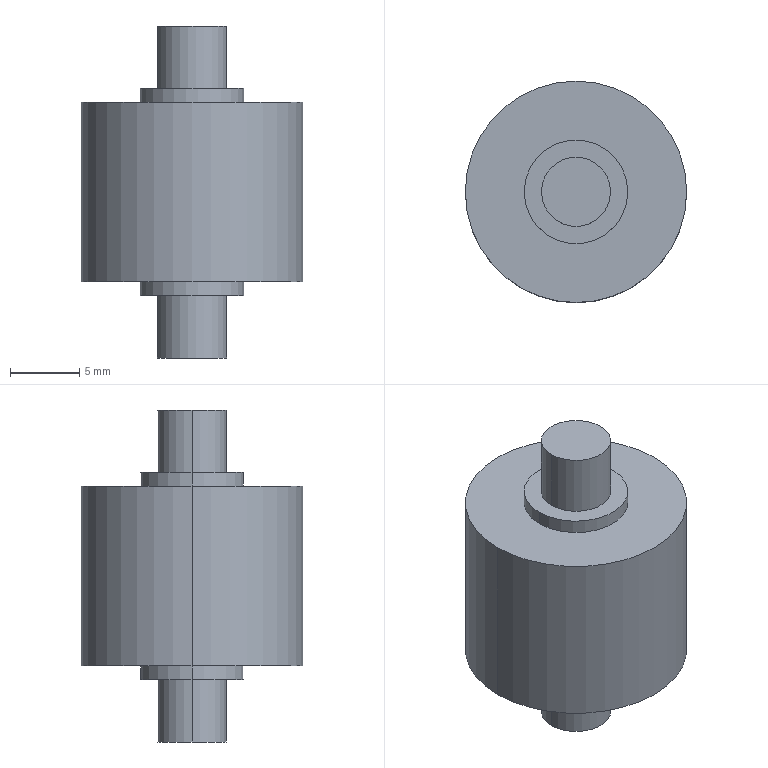Part | 1 solid | 16 faces | box 16 x 16 x 24 mm | volume 2879 mm3 | cylinder 10 | plane 6 | commonest cylinder face diameters 5 x4 7.5 x4 16 x2
STEP:
#1=CARTESIAN_POINT('',(2.5,0.,12.));
#2=VERTEX_POINT('',#1);
#3=CARTESIAN_POINT('',(-2.5,0.,12.));
#4=VERTEX_POINT('',#3);
#5=CARTESIAN_POINT('',(0.,0.,12.));
#6=DIRECTION('',(0.,0.,1.));
#7=DIRECTION('',(1.,0.,0.));
#8=AXIS2_PLACEMENT_3D('',#5,#6,#7);
#9=CIRCLE('',#8,2.5);
#10=EDGE_CURVE('',#2,#4,#9,.T.);
#11=ORIENTED_EDGE('',*,*,#10,.F.);
#12=CARTESIAN_POINT('',(2.5,0.,7.5));
#13=VERTEX_POINT('',#12);
#14=CARTESIAN_POINT('',(2.5,0.,12.));
#15=DIRECTION('',(0.,0.,-1.));
#16=VECTOR('',#15,1000.);
#17=LINE('',#14,#16);
#18=EDGE_CURVE('',#2,#13,#17,.T.);
#19=ORIENTED_EDGE('',*,*,#18,.T.);
#20=CARTESIAN_POINT('',(-2.5,0.,7.5));
#21=VERTEX_POINT('',#20);
#22=CARTESIAN_POINT('',(0.,0.,7.5));
#23=DIRECTION('',(0.,0.,1.));
#24=DIRECTION('',(1.,0.,0.));
#25=AXIS2_PLACEMENT_3D('',#22,#23,#24);
#26=CIRCLE('',#25,2.5);
#27=EDGE_CURVE('',#13,#21,#26,.T.);
#28=ORIENTED_EDGE('',*,*,#27,.T.);
#29=CARTESIAN_POINT('',(-2.5,0.,12.));
#30=DIRECTION('',(0.,0.,-1.));
#31=VECTOR('',#30,1000.);
#32=LINE('',#29,#31);
#33=EDGE_CURVE('',#4,#21,#32,.T.);
#34=ORIENTED_EDGE('',*,*,#33,.F.);
#35=EDGE_LOOP('',(#11,#19,#28,#34));
#36=FACE_OUTER_BOUND('',#35,.T.);
#37=CARTESIAN_POINT('',(0.,0.,12.));
#38=DIRECTION('',(0.,0.,-1.));
#39=DIRECTION('',(-1.,0.,0.));
#40=AXIS2_PLACEMENT_3D('',#37,#38,#39);
#41=CYLINDRICAL_SURFACE('',#40,2.5);
#42=ADVANCED_FACE('',(#36),#41,.T.);
#43=CARTESIAN_POINT('',(3.75,0.,7.5));
#44=VERTEX_POINT('',#43);
#45=CARTESIAN_POINT('',(-3.75,0.,7.5));
#46=VERTEX_POINT('',#45);
#47=CARTESIAN_POINT('',(0.,0.,7.5));
#48=DIRECTION('',(0.,0.,1.));
#49=DIRECTION('',(1.,0.,0.));
#50=AXIS2_PLACEMENT_3D('',#47,#48,#49);
#51=CIRCLE('',#50,3.75);
#52=EDGE_CURVE('',#44,#46,#51,.T.);
#53=ORIENTED_EDGE('',*,*,#52,.F.);
#54=CARTESIAN_POINT('',(3.75,0.,6.5));
#55=VERTEX_POINT('',#54);
#56=CARTESIAN_POINT('',(3.75,0.,7.5));
#57=DIRECTION('',(0.,0.,-1.));
#58=VECTOR('',#57,1000.);
#59=LINE('',#56,#58);
#60=EDGE_CURVE('',#44,#55,#59,.T.);
#61=ORIENTED_EDGE('',*,*,#60,.T.);
#62=CARTESIAN_POINT('',(-3.75,0.,6.5));
#63=VERTEX_POINT('',#62);
#64=CARTESIAN_POINT('',(0.,0.,6.5));
#65=DIRECTION('',(0.,0.,1.));
#66=DIRECTION('',(1.,0.,0.));
#67=AXIS2_PLACEMENT_3D('',#64,#65,#66);
#68=CIRCLE('',#67,3.75);
#69=EDGE_CURVE('',#55,#63,#68,.T.);
#70=ORIENTED_EDGE('',*,*,#69,.T.);
#71=CARTESIAN_POINT('',(-3.75,0.,7.5));
#72=DIRECTION('',(0.,0.,-1.));
#73=VECTOR('',#72,1000.);
#74=LINE('',#71,#73);
#75=EDGE_CURVE('',#46,#63,#74,.T.);
#76=ORIENTED_EDGE('',*,*,#75,.F.);
#77=EDGE_LOOP('',(#53,#61,#70,#76));
#78=FACE_OUTER_BOUND('',#77,.T.);
#79=CARTESIAN_POINT('',(0.,0.,7.5));
#80=DIRECTION('',(0.,0.,-1.));
#81=DIRECTION('',(-1.,0.,0.));
#82=AXIS2_PLACEMENT_3D('',#79,#80,#81);
#83=CYLINDRICAL_SURFACE('',#82,3.75);
#84=ADVANCED_FACE('',(#78),#83,.T.);
#85=CARTESIAN_POINT('',(-2.5,0.,-7.5));
#86=VERTEX_POINT('',#85);
#87=CARTESIAN_POINT('',(2.5,0.,-7.5));
#88=VERTEX_POINT('',#87);
#89=CARTESIAN_POINT('',(0.,0.,-7.5));
#90=DIRECTION('',(0.,0.,-1.));
#91=DIRECTION('',(-1.,0.,0.));
#92=AXIS2_PLACEMENT_3D('',#89,#90,#91);
#93=CIRCLE('',#92,2.5);
#94=EDGE_CURVE('',#86,#88,#93,.T.);
#95=ORIENTED_EDGE('',*,*,#94,.T.);
#96=CARTESIAN_POINT('',(2.5,0.,-12.));
#97=VERTEX_POINT('',#96);
#98=CARTESIAN_POINT('',(2.5,0.,12.));
#99=DIRECTION('',(0.,0.,-1.));
#100=VECTOR('',#99,1000.);
#101=LINE('',#98,#100);
#102=EDGE_CURVE('',#88,#97,#101,.T.);
#103=ORIENTED_EDGE('',*,*,#102,.T.);
#104=CARTESIAN_POINT('',(-2.5,0.,-12.));
#105=VERTEX_POINT('',#104);
#106=CARTESIAN_POINT('',(0.,0.,-12.));
#107=DIRECTION('',(0.,0.,1.));
#108=DIRECTION('',(1.,0.,0.));
#109=AXIS2_PLACEMENT_3D('',#106,#107,#108);
#110=CIRCLE('',#109,2.5);
#111=EDGE_CURVE('',#97,#105,#110,.T.);
#112=ORIENTED_EDGE('',*,*,#111,.T.);
#113=CARTESIAN_POINT('',(-2.5,0.,12.));
#114=DIRECTION('',(0.,0.,-1.));
#115=VECTOR('',#114,1000.);
#116=LINE('',#113,#115);
#117=EDGE_CURVE('',#86,#105,#116,.T.);
#118=ORIENTED_EDGE('',*,*,#117,.F.);
#119=EDGE_LOOP('',(#95,#103,#112,#118));
#120=FACE_OUTER_BOUND('',#119,.T.);
#121=CARTESIAN_POINT('',(0.,0.,12.));
#122=DIRECTION('',(0.,0.,-1.));
#123=DIRECTION('',(-1.,0.,0.));
#124=AXIS2_PLACEMENT_3D('',#121,#122,#123);
#125=CYLINDRICAL_SURFACE('',#124,2.5);
#126=ADVANCED_FACE('',(#120),#125,.T.);
#127=CARTESIAN_POINT('',(-3.75,0.,-7.5));
#128=VERTEX_POINT('',#127);
#129=CARTESIAN_POINT('',(3.75,0.,-7.5));
#130=VERTEX_POINT('',#129);
#131=CARTESIAN_POINT('',(0.,0.,-7.5));
#132=DIRECTION('',(0.,0.,-1.));
#133=DIRECTION('',(-1.,0.,0.));
#134=AXIS2_PLACEMENT_3D('',#131,#132,#133);
#135=CIRCLE('',#134,3.75);
#136=EDGE_CURVE('',#128,#130,#135,.T.);
#137=ORIENTED_EDGE('',*,*,#136,.F.);
#138=CARTESIAN_POINT('',(-3.75,0.,-6.5));
#139=VERTEX_POINT('',#138);
#140=CARTESIAN_POINT('',(-3.75,0.,-7.5));
#141=DIRECTION('',(0.,0.,1.));
#142=VECTOR('',#141,1000.);
#143=LINE('',#140,#142);
#144=EDGE_CURVE('',#128,#139,#143,.T.);
#145=ORIENTED_EDGE('',*,*,#144,.T.);
#146=CARTESIAN_POINT('',(3.75,0.,-6.5));
#147=VERTEX_POINT('',#146);
#148=CARTESIAN_POINT('',(0.,0.,-6.5));
#149=DIRECTION('',(0.,0.,-1.));
#150=DIRECTION('',(1.,0.,0.));
#151=AXIS2_PLACEMENT_3D('',#148,#149,#150);
#152=CIRCLE('',#151,3.75);
#153=EDGE_CURVE('',#139,#147,#152,.T.);
#154=ORIENTED_EDGE('',*,*,#153,.T.);
#155=CARTESIAN_POINT('',(3.75,0.,-7.5));
#156=DIRECTION('',(0.,0.,1.));
#157=VECTOR('',#156,1000.);
#158=LINE('',#155,#157);
#159=EDGE_CURVE('',#130,#147,#158,.T.);
#160=ORIENTED_EDGE('',*,*,#159,.F.);
#161=EDGE_LOOP('',(#137,#145,#154,#160));
#162=FACE_OUTER_BOUND('',#161,.T.);
#163=CARTESIAN_POINT('',(0.,0.,-7.5));
#164=DIRECTION('',(0.,0.,1.));
#165=DIRECTION('',(1.,0.,0.));
#166=AXIS2_PLACEMENT_3D('',#163,#164,#165);
#167=CYLINDRICAL_SURFACE('',#166,3.75);
#168=ADVANCED_FACE('',(#162),#167,.T.);
#169=CARTESIAN_POINT('',(8.,0.,6.5));
#170=VERTEX_POINT('',#169);
#171=CARTESIAN_POINT('',(-8.,0.,6.5));
#172=VERTEX_POINT('',#171);
#173=CARTESIAN_POINT('',(0.,0.,6.5));
#174=DIRECTION('',(0.,0.,1.));
#175=DIRECTION('',(1.,0.,0.));
#176=AXIS2_PLACEMENT_3D('',#173,#174,#175);
#177=CIRCLE('',#176,8.);
#178=EDGE_CURVE('',#170,#172,#177,.T.);
#179=ORIENTED_EDGE('',*,*,#178,.F.);
#180=CARTESIAN_POINT('',(8.,0.,-6.5));
#181=VERTEX_POINT('',#180);
#182=CARTESIAN_POINT('',(8.,0.,6.5));
#183=DIRECTION('',(0.,0.,-1.));
#184=VECTOR('',#183,1000.);
#185=LINE('',#182,#184);
#186=EDGE_CURVE('',#170,#181,#185,.T.);
#187=ORIENTED_EDGE('',*,*,#186,.T.);
#188=CARTESIAN_POINT('',(-8.,0.,-6.5));
#189=VERTEX_POINT('',#188);
#190=CARTESIAN_POINT('',(0.,0.,-6.5));
#191=DIRECTION('',(0.,0.,1.));
#192=DIRECTION('',(1.,0.,0.));
#193=AXIS2_PLACEMENT_3D('',#190,#191,#192);
#194=CIRCLE('',#193,8.);
#195=EDGE_CURVE('',#181,#189,#194,.T.);
#196=ORIENTED_EDGE('',*,*,#195,.T.);
#197=CARTESIAN_POINT('',(-8.,0.,6.5));
#198=DIRECTION('',(0.,0.,-1.));
#199=VECTOR('',#198,1000.);
#200=LINE('',#197,#199);
#201=EDGE_CURVE('',#172,#189,#200,.T.);
#202=ORIENTED_EDGE('',*,*,#201,.F.);
#203=EDGE_LOOP('',(#179,#187,#196,#202));
#204=FACE_OUTER_BOUND('',#203,.T.);
#205=CARTESIAN_POINT('',(0.,0.,6.5));
#206=DIRECTION('',(0.,0.,-1.));
#207=DIRECTION('',(-1.,0.,0.));
#208=AXIS2_PLACEMENT_3D('',#205,#206,#207);
#209=CYLINDRICAL_SURFACE('',#208,8.);
#210=ADVANCED_FACE('',(#204),#209,.T.);
#211=ORIENTED_EDGE('',*,*,#186,.F.);
#212=CARTESIAN_POINT('',(0.,0.,6.5));
#213=DIRECTION('',(0.,0.,1.));
#214=DIRECTION('',(1.,0.,0.));
#215=AXIS2_PLACEMENT_3D('',#212,#213,#214);
#216=CIRCLE('',#215,8.);
#217=EDGE_CURVE('',#172,#170,#216,.T.);
#218=ORIENTED_EDGE('',*,*,#217,.F.);
#219=ORIENTED_EDGE('',*,*,#201,.T.);
#220=CARTESIAN_POINT('',(0.,0.,-6.5));
#221=DIRECTION('',(0.,0.,1.));
#222=DIRECTION('',(1.,0.,0.));
#223=AXIS2_PLACEMENT_3D('',#220,#221,#222);
#224=CIRCLE('',#223,8.);
#225=EDGE_CURVE('',#189,#181,#224,.T.);
#226=ORIENTED_EDGE('',*,*,#225,.T.);
#227=EDGE_LOOP('',(#211,#218,#219,#226));
#228=FACE_OUTER_BOUND('',#227,.T.);
#229=CARTESIAN_POINT('',(0.,0.,6.5));
#230=DIRECTION('',(0.,0.,-1.));
#231=DIRECTION('',(-1.,0.,0.));
#232=AXIS2_PLACEMENT_3D('',#229,#230,#231);
#233=CYLINDRICAL_SURFACE('',#232,8.);
#234=ADVANCED_FACE('',(#228),#233,.T.);
#235=CARTESIAN_POINT('',(0.,0.,6.5));
#236=DIRECTION('',(0.,0.,1.));
#237=DIRECTION('',(1.,0.,0.));
#238=AXIS2_PLACEMENT_3D('',#235,#236,#237);
#239=CIRCLE('',#238,3.75);
#240=EDGE_CURVE('',#63,#55,#239,.T.);
#241=ORIENTED_EDGE('',*,*,#240,.F.);
#242=ORIENTED_EDGE('',*,*,#69,.F.);
#243=EDGE_LOOP('',(#241,#242));
#244=FACE_BOUND('',#243,.T.);
#245=ORIENTED_EDGE('',*,*,#217,.T.);
#246=ORIENTED_EDGE('',*,*,#178,.T.);
#247=EDGE_LOOP('',(#245,#246));
#248=FACE_OUTER_BOUND('',#247,.T.);
#249=CARTESIAN_POINT('',(0.,0.,6.5));
#250=DIRECTION('',(0.,0.,1.));
#251=DIRECTION('',(1.,0.,0.));
#252=AXIS2_PLACEMENT_3D('',#249,#250,#251);
#253=PLANE('',#252);
#254=ADVANCED_FACE('',(#244,#248),#253,.T.);
#255=CARTESIAN_POINT('',(0.,0.,-6.5));
#256=DIRECTION('',(0.,0.,-1.));
#257=DIRECTION('',(1.,0.,0.));
#258=AXIS2_PLACEMENT_3D('',#255,#256,#257);
#259=CIRCLE('',#258,3.75);
#260=EDGE_CURVE('',#147,#139,#259,.T.);
#261=ORIENTED_EDGE('',*,*,#260,.F.);
#262=ORIENTED_EDGE('',*,*,#153,.F.);
#263=EDGE_LOOP('',(#261,#262));
#264=FACE_BOUND('',#263,.T.);
#265=ORIENTED_EDGE('',*,*,#225,.F.);
#266=ORIENTED_EDGE('',*,*,#195,.F.);
#267=EDGE_LOOP('',(#265,#266));
#268=FACE_OUTER_BOUND('',#267,.T.);
#269=CARTESIAN_POINT('',(0.,0.,-6.5));
#270=DIRECTION('',(0.,0.,1.));
#271=DIRECTION('',(1.,0.,0.));
#272=AXIS2_PLACEMENT_3D('',#269,#270,#271);
#273=PLANE('',#272);
#274=ADVANCED_FACE('',(#264,#268),#273,.F.);
#275=ORIENTED_EDGE('',*,*,#144,.F.);
#276=CARTESIAN_POINT('',(0.,0.,-7.5));
#277=DIRECTION('',(0.,0.,-1.));
#278=DIRECTION('',(-1.,0.,0.));
#279=AXIS2_PLACEMENT_3D('',#276,#277,#278);
#280=CIRCLE('',#279,3.75);
#281=EDGE_CURVE('',#130,#128,#280,.T.);
#282=ORIENTED_EDGE('',*,*,#281,.F.);
#283=ORIENTED_EDGE('',*,*,#159,.T.);
#284=ORIENTED_EDGE('',*,*,#260,.T.);
#285=EDGE_LOOP('',(#275,#282,#283,#284));
#286=FACE_OUTER_BOUND('',#285,.T.);
#287=CARTESIAN_POINT('',(0.,0.,-7.5));
#288=DIRECTION('',(0.,0.,1.));
#289=DIRECTION('',(1.,0.,0.));
#290=AXIS2_PLACEMENT_3D('',#287,#288,#289);
#291=CYLINDRICAL_SURFACE('',#290,3.75);
#292=ADVANCED_FACE('',(#286),#291,.T.);
#293=ORIENTED_EDGE('',*,*,#94,.F.);
#294=CARTESIAN_POINT('',(0.,0.,-7.5));
#295=DIRECTION('',(0.,0.,-1.));
#296=DIRECTION('',(-1.,0.,0.));
#297=AXIS2_PLACEMENT_3D('',#294,#295,#296);
#298=CIRCLE('',#297,2.5);
#299=EDGE_CURVE('',#88,#86,#298,.T.);
#300=ORIENTED_EDGE('',*,*,#299,.F.);
#301=EDGE_LOOP('',(#293,#300));
#302=FACE_BOUND('',#301,.T.);
#303=ORIENTED_EDGE('',*,*,#281,.T.);
#304=ORIENTED_EDGE('',*,*,#136,.T.);
#305=EDGE_LOOP('',(#303,#304));
#306=FACE_OUTER_BOUND('',#305,.T.);
#307=CARTESIAN_POINT('',(0.,0.,-7.5));
#308=DIRECTION('',(0.,0.,-1.));
#309=DIRECTION('',(-1.,0.,0.));
#310=AXIS2_PLACEMENT_3D('',#307,#308,#309);
#311=PLANE('',#310);
#312=ADVANCED_FACE('',(#302,#306),#311,.T.);
#313=CARTESIAN_POINT('',(0.,0.,-12.));
#314=DIRECTION('',(0.,0.,1.));
#315=DIRECTION('',(1.,0.,0.));
#316=AXIS2_PLACEMENT_3D('',#313,#314,#315);
#317=CIRCLE('',#316,2.5);
#318=EDGE_CURVE('',#105,#97,#317,.T.);
#319=ORIENTED_EDGE('',*,*,#318,.F.);
#320=ORIENTED_EDGE('',*,*,#111,.F.);
#321=EDGE_LOOP('',(#319,#320));
#322=FACE_OUTER_BOUND('',#321,.T.);
#323=CARTESIAN_POINT('',(0.,0.,-12.));
#324=DIRECTION('',(0.,0.,1.));
#325=DIRECTION('',(1.,0.,0.));
#326=AXIS2_PLACEMENT_3D('',#323,#324,#325);
#327=PLANE('',#326);
#328=ADVANCED_FACE('',(#322),#327,.F.);
#329=ORIENTED_EDGE('',*,*,#102,.F.);
#330=ORIENTED_EDGE('',*,*,#299,.T.);
#331=ORIENTED_EDGE('',*,*,#117,.T.);
#332=ORIENTED_EDGE('',*,*,#318,.T.);
#333=EDGE_LOOP('',(#329,#330,#331,#332));
#334=FACE_OUTER_BOUND('',#333,.T.);
#335=CARTESIAN_POINT('',(0.,0.,12.));
#336=DIRECTION('',(0.,0.,-1.));
#337=DIRECTION('',(-1.,0.,0.));
#338=AXIS2_PLACEMENT_3D('',#335,#336,#337);
#339=CYLINDRICAL_SURFACE('',#338,2.5);
#340=ADVANCED_FACE('',(#334),#339,.T.);
#341=ORIENTED_EDGE('',*,*,#60,.F.);
#342=CARTESIAN_POINT('',(0.,0.,7.5));
#343=DIRECTION('',(0.,0.,1.));
#344=DIRECTION('',(1.,0.,0.));
#345=AXIS2_PLACEMENT_3D('',#342,#343,#344);
#346=CIRCLE('',#345,3.75);
#347=EDGE_CURVE('',#46,#44,#346,.T.);
#348=ORIENTED_EDGE('',*,*,#347,.F.);
#349=ORIENTED_EDGE('',*,*,#75,.T.);
#350=ORIENTED_EDGE('',*,*,#240,.T.);
#351=EDGE_LOOP('',(#341,#348,#349,#350));
#352=FACE_OUTER_BOUND('',#351,.T.);
#353=CARTESIAN_POINT('',(0.,0.,7.5));
#354=DIRECTION('',(0.,0.,-1.));
#355=DIRECTION('',(-1.,0.,0.));
#356=AXIS2_PLACEMENT_3D('',#353,#354,#355);
#357=CYLINDRICAL_SURFACE('',#356,3.75);
#358=ADVANCED_FACE('',(#352),#357,.T.);
#359=CARTESIAN_POINT('',(0.,0.,7.5));
#360=DIRECTION('',(0.,0.,1.));
#361=DIRECTION('',(1.,0.,0.));
#362=AXIS2_PLACEMENT_3D('',#359,#360,#361);
#363=CIRCLE('',#362,2.5);
#364=EDGE_CURVE('',#21,#13,#363,.T.);
#365=ORIENTED_EDGE('',*,*,#364,.F.);
#366=ORIENTED_EDGE('',*,*,#27,.F.);
#367=EDGE_LOOP('',(#365,#366));
#368=FACE_BOUND('',#367,.T.);
#369=ORIENTED_EDGE('',*,*,#347,.T.);
#370=ORIENTED_EDGE('',*,*,#52,.T.);
#371=EDGE_LOOP('',(#369,#370));
#372=FACE_OUTER_BOUND('',#371,.T.);
#373=CARTESIAN_POINT('',(0.,0.,7.5));
#374=DIRECTION('',(0.,0.,1.));
#375=DIRECTION('',(1.,0.,0.));
#376=AXIS2_PLACEMENT_3D('',#373,#374,#375);
#377=PLANE('',#376);
#378=ADVANCED_FACE('',(#368,#372),#377,.T.);
#379=CARTESIAN_POINT('',(0.,0.,12.));
#380=DIRECTION('',(0.,0.,1.));
#381=DIRECTION('',(1.,0.,0.));
#382=AXIS2_PLACEMENT_3D('',#379,#380,#381);
#383=CIRCLE('',#382,2.5);
#384=EDGE_CURVE('',#4,#2,#383,.T.);
#385=ORIENTED_EDGE('',*,*,#384,.T.);
#386=ORIENTED_EDGE('',*,*,#10,.T.);
#387=EDGE_LOOP('',(#385,#386));
#388=FACE_OUTER_BOUND('',#387,.T.);
#389=CARTESIAN_POINT('',(0.,0.,12.));
#390=DIRECTION('',(0.,0.,1.));
#391=DIRECTION('',(1.,0.,0.));
#392=AXIS2_PLACEMENT_3D('',#389,#390,#391);
#393=PLANE('',#392);
#394=ADVANCED_FACE('',(#388),#393,.T.);
#395=ORIENTED_EDGE('',*,*,#18,.F.);
#396=ORIENTED_EDGE('',*,*,#384,.F.);
#397=ORIENTED_EDGE('',*,*,#33,.T.);
#398=ORIENTED_EDGE('',*,*,#364,.T.);
#399=EDGE_LOOP('',(#395,#396,#397,#398));
#400=FACE_OUTER_BOUND('',#399,.T.);
#401=CARTESIAN_POINT('',(0.,0.,12.));
#402=DIRECTION('',(0.,0.,-1.));
#403=DIRECTION('',(-1.,0.,0.));
#404=AXIS2_PLACEMENT_3D('',#401,#402,#403);
#405=CYLINDRICAL_SURFACE('',#404,2.5);
#406=ADVANCED_FACE('',(#400),#405,.T.);
#407=CLOSED_SHELL('',(#42,#84,#126,#168,#210,#234,#254,#274,#292,#312,#328,#340,#358,#378,#394,#406));
#408=MANIFOLD_SOLID_BREP('',#407);
#409=CARTESIAN_POINT('',(0.,0.,0.));
#410=DIRECTION('',(0.,0.,1.));
#411=DIRECTION('',(1.,0.,0.));
#412=AXIS2_PLACEMENT_3D('',#409,#410,#411);
#413=(LENGTH_UNIT()NAMED_UNIT(*)SI_UNIT(.MILLI.,.METRE.));
#414=UNCERTAINTY_MEASURE_WITH_UNIT(LENGTH_MEASURE(0.00001),#413,'','');
#415=(NAMED_UNIT(*)PLANE_ANGLE_UNIT()SI_UNIT($,.RADIAN.));
#416=(NAMED_UNIT(*)SI_UNIT($,.STERADIAN.)SOLID_ANGLE_UNIT());
#417=(GEOMETRIC_REPRESENTATION_CONTEXT(3)GLOBAL_UNCERTAINTY_ASSIGNED_CONTEXT((#414))GLOBAL_UNIT_ASSIGNED_CONTEXT((#413,#415,#416))REPRESENTATION_CONTEXT('',''));
#418=ADVANCED_BREP_SHAPE_REPRESENTATION('',(#408,#412),#417);